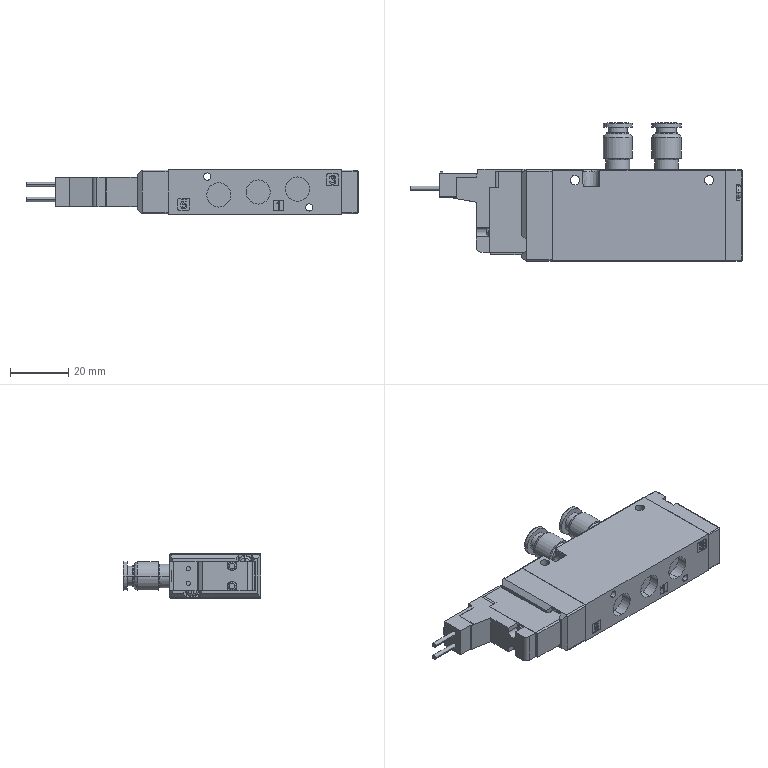Part | STEP file | 4RD219-GS4-E2-3_default | 13 solids | 686 faces | box 113.84 x 47.304 x 15.298 mm | volume 40312 mm3 | plane 320 | cylinder 223 | spline 90 | cone 53 | commonest cylinder face diameters 0.6 x44 2.5 x20 8.3 x10 1 x8 2.208 x8 2.6 x8